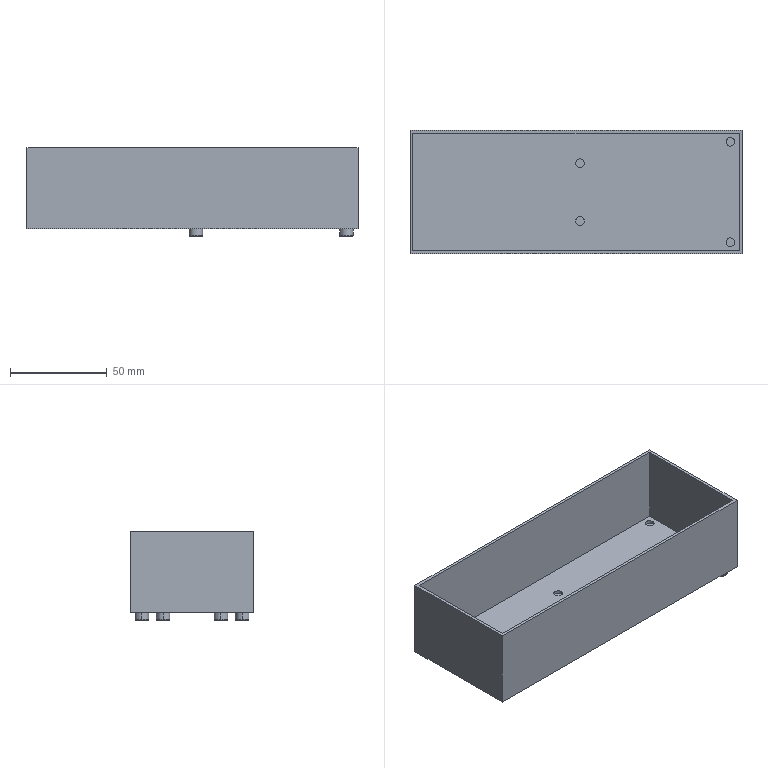Part | SolidWorks | features BaseBody 1 | 1 solid | 71 faces | box 172 x 64 x 46 mm | volume 45275 mm3 | plane 47 | cylinder 16 | spline 8 | commonest cylinder face diameters 4.5 x8 7 x8